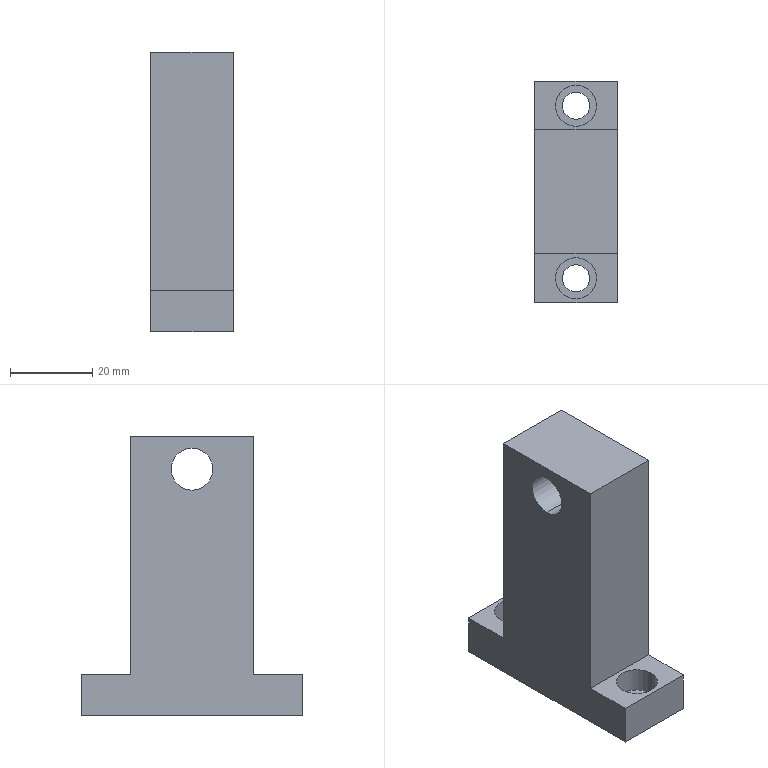Part | SolidWorks | features HoleWzd 2, Extrusion 1, ICE 1 | 1 solid | 22 faces | box 20 x 54 x 68 mm | volume 42750 mm3 | plane 12 | cylinder 10 | commonest cylinder face diameters 6.6 x4 10 x4 10.2 x2
STEP:
#1=CARTESIAN_POINT('',(-16.388,2.618,65.1));
#2=VERTEX_POINT('',#1);
#3=CARTESIAN_POINT('',(-16.388,2.618,54.9));
#4=VERTEX_POINT('',#3);
#5=CARTESIAN_POINT('',(-16.388,2.618,60.));
#6=DIRECTION('',(1.,0.,0.));
#7=DIRECTION('',(0.,1.,0.));
#8=AXIS2_PLACEMENT_3D('',#5,#6,#7);
#9=CIRCLE('',#8,5.1);
#10=EDGE_CURVE('',#2,#4,#9,.T.);
#11=ORIENTED_EDGE('',*,*,#10,.T.);
#12=CARTESIAN_POINT('',(-36.388,2.618,54.9));
#13=VERTEX_POINT('',#12);
#14=CARTESIAN_POINT('',(-36.388,2.618,54.9));
#15=DIRECTION('',(-1.,0.,0.));
#16=VECTOR('',#15,1000.);
#17=LINE('',#14,#16);
#18=EDGE_CURVE('',#4,#13,#17,.T.);
#19=ORIENTED_EDGE('',*,*,#18,.T.);
#20=CARTESIAN_POINT('',(-36.388,2.618,65.1));
#21=VERTEX_POINT('',#20);
#22=CARTESIAN_POINT('',(-36.388,2.618,60.));
#23=DIRECTION('',(-1.,0.,0.));
#24=DIRECTION('',(0.,0.,1.));
#25=AXIS2_PLACEMENT_3D('',#22,#23,#24);
#26=CIRCLE('',#25,5.1);
#27=EDGE_CURVE('',#13,#21,#26,.T.);
#28=ORIENTED_EDGE('',*,*,#27,.T.);
#29=CARTESIAN_POINT('',(-36.388,2.618,65.1));
#30=DIRECTION('',(-1.,0.,0.));
#31=VECTOR('',#30,1000.);
#32=LINE('',#29,#31);
#33=EDGE_CURVE('',#2,#21,#32,.T.);
#34=ORIENTED_EDGE('',*,*,#33,.F.);
#35=EDGE_LOOP('',(#11,#19,#28,#34));
#36=FACE_OUTER_BOUND('',#35,.T.);
#37=CARTESIAN_POINT('',(-36.388,2.618,60.));
#38=DIRECTION('',(-1.,0.,0.));
#39=DIRECTION('',(0.,0.,1.));
#40=AXIS2_PLACEMENT_3D('',#37,#38,#39);
#41=CYLINDRICAL_SURFACE('',#40,5.1);
#42=ADVANCED_FACE('',(#36),#41,.F.);
#43=CARTESIAN_POINT('',(-31.388,23.618,4.));
#44=VERTEX_POINT('',#43);
#45=CARTESIAN_POINT('',(-21.388,23.618,4.));
#46=VERTEX_POINT('',#45);
#47=CARTESIAN_POINT('',(-26.388,23.618,4.));
#48=DIRECTION('',(0.,0.,1.));
#49=DIRECTION('',(1.,0.,0.));
#50=AXIS2_PLACEMENT_3D('',#47,#48,#49);
#51=CIRCLE('',#50,5.);
#52=EDGE_CURVE('',#44,#46,#51,.T.);
#53=ORIENTED_EDGE('',*,*,#52,.F.);
#54=CARTESIAN_POINT('',(-31.388,23.618,10.));
#55=VERTEX_POINT('',#54);
#56=CARTESIAN_POINT('',(-31.388,23.618,10.));
#57=DIRECTION('',(0.,0.,1.));
#58=VECTOR('',#57,1000.);
#59=LINE('',#56,#58);
#60=EDGE_CURVE('',#44,#55,#59,.T.);
#61=ORIENTED_EDGE('',*,*,#60,.T.);
#62=CARTESIAN_POINT('',(-21.388,23.618,10.));
#63=VERTEX_POINT('',#62);
#64=CARTESIAN_POINT('',(-26.388,23.618,10.));
#65=DIRECTION('',(0.,0.,1.));
#66=DIRECTION('',(1.,0.,0.));
#67=AXIS2_PLACEMENT_3D('',#64,#65,#66);
#68=CIRCLE('',#67,5.);
#69=EDGE_CURVE('',#55,#63,#68,.T.);
#70=ORIENTED_EDGE('',*,*,#69,.T.);
#71=CARTESIAN_POINT('',(-21.388,23.618,10.));
#72=DIRECTION('',(0.,0.,1.));
#73=VECTOR('',#72,1000.);
#74=LINE('',#71,#73);
#75=EDGE_CURVE('',#46,#63,#74,.T.);
#76=ORIENTED_EDGE('',*,*,#75,.F.);
#77=EDGE_LOOP('',(#53,#61,#70,#76));
#78=FACE_OUTER_BOUND('',#77,.T.);
#79=CARTESIAN_POINT('',(-26.388,23.618,10.));
#80=DIRECTION('',(0.,0.,1.));
#81=DIRECTION('',(1.,0.,0.));
#82=AXIS2_PLACEMENT_3D('',#79,#80,#81);
#83=CYLINDRICAL_SURFACE('',#82,5.);
#84=ADVANCED_FACE('',(#78),#83,.F.);
#85=CARTESIAN_POINT('',(-29.688,23.618,0.));
#86=VERTEX_POINT('',#85);
#87=CARTESIAN_POINT('',(-23.088,23.618,0.));
#88=VERTEX_POINT('',#87);
#89=CARTESIAN_POINT('',(-26.388,23.618,0.));
#90=DIRECTION('',(0.,0.,1.));
#91=DIRECTION('',(1.,0.,0.));
#92=AXIS2_PLACEMENT_3D('',#89,#90,#91);
#93=CIRCLE('',#92,3.3);
#94=EDGE_CURVE('',#86,#88,#93,.T.);
#95=ORIENTED_EDGE('',*,*,#94,.F.);
#96=CARTESIAN_POINT('',(-29.688,23.618,4.));
#97=VERTEX_POINT('',#96);
#98=CARTESIAN_POINT('',(-29.688,23.618,10.));
#99=DIRECTION('',(0.,0.,1.));
#100=VECTOR('',#99,1000.);
#101=LINE('',#98,#100);
#102=EDGE_CURVE('',#86,#97,#101,.T.);
#103=ORIENTED_EDGE('',*,*,#102,.T.);
#104=CARTESIAN_POINT('',(-23.088,23.618,4.));
#105=VERTEX_POINT('',#104);
#106=CARTESIAN_POINT('',(-26.388,23.618,4.));
#107=DIRECTION('',(0.,0.,1.));
#108=DIRECTION('',(1.,0.,0.));
#109=AXIS2_PLACEMENT_3D('',#106,#107,#108);
#110=CIRCLE('',#109,3.3);
#111=EDGE_CURVE('',#97,#105,#110,.T.);
#112=ORIENTED_EDGE('',*,*,#111,.T.);
#113=CARTESIAN_POINT('',(-23.088,23.618,10.));
#114=DIRECTION('',(0.,0.,1.));
#115=VECTOR('',#114,1000.);
#116=LINE('',#113,#115);
#117=EDGE_CURVE('',#88,#105,#116,.T.);
#118=ORIENTED_EDGE('',*,*,#117,.F.);
#119=EDGE_LOOP('',(#95,#103,#112,#118));
#120=FACE_OUTER_BOUND('',#119,.T.);
#121=CARTESIAN_POINT('',(-26.388,23.618,10.));
#122=DIRECTION('',(0.,0.,1.));
#123=DIRECTION('',(1.,0.,0.));
#124=AXIS2_PLACEMENT_3D('',#121,#122,#123);
#125=CYLINDRICAL_SURFACE('',#124,3.3);
#126=ADVANCED_FACE('',(#120),#125,.F.);
#127=CARTESIAN_POINT('',(-31.388,-18.382,4.));
#128=VERTEX_POINT('',#127);
#129=CARTESIAN_POINT('',(-21.388,-18.382,4.));
#130=VERTEX_POINT('',#129);
#131=CARTESIAN_POINT('',(-26.388,-18.382,4.));
#132=DIRECTION('',(0.,0.,1.));
#133=DIRECTION('',(1.,0.,0.));
#134=AXIS2_PLACEMENT_3D('',#131,#132,#133);
#135=CIRCLE('',#134,5.);
#136=EDGE_CURVE('',#128,#130,#135,.T.);
#137=ORIENTED_EDGE('',*,*,#136,.F.);
#138=CARTESIAN_POINT('',(-31.388,-18.382,10.));
#139=VERTEX_POINT('',#138);
#140=CARTESIAN_POINT('',(-31.388,-18.382,10.));
#141=DIRECTION('',(0.,0.,1.));
#142=VECTOR('',#141,1000.);
#143=LINE('',#140,#142);
#144=EDGE_CURVE('',#128,#139,#143,.T.);
#145=ORIENTED_EDGE('',*,*,#144,.T.);
#146=CARTESIAN_POINT('',(-21.388,-18.382,10.));
#147=VERTEX_POINT('',#146);
#148=CARTESIAN_POINT('',(-26.388,-18.382,10.));
#149=DIRECTION('',(0.,0.,1.));
#150=DIRECTION('',(1.,0.,0.));
#151=AXIS2_PLACEMENT_3D('',#148,#149,#150);
#152=CIRCLE('',#151,5.);
#153=EDGE_CURVE('',#139,#147,#152,.T.);
#154=ORIENTED_EDGE('',*,*,#153,.T.);
#155=CARTESIAN_POINT('',(-21.388,-18.382,10.));
#156=DIRECTION('',(0.,0.,1.));
#157=VECTOR('',#156,1000.);
#158=LINE('',#155,#157);
#159=EDGE_CURVE('',#130,#147,#158,.T.);
#160=ORIENTED_EDGE('',*,*,#159,.F.);
#161=EDGE_LOOP('',(#137,#145,#154,#160));
#162=FACE_OUTER_BOUND('',#161,.T.);
#163=CARTESIAN_POINT('',(-26.388,-18.382,10.));
#164=DIRECTION('',(0.,0.,1.));
#165=DIRECTION('',(1.,0.,0.));
#166=AXIS2_PLACEMENT_3D('',#163,#164,#165);
#167=CYLINDRICAL_SURFACE('',#166,5.);
#168=ADVANCED_FACE('',(#162),#167,.F.);
#169=CARTESIAN_POINT('',(-29.688,-18.382,0.));
#170=VERTEX_POINT('',#169);
#171=CARTESIAN_POINT('',(-23.088,-18.382,0.));
#172=VERTEX_POINT('',#171);
#173=CARTESIAN_POINT('',(-26.388,-18.382,0.));
#174=DIRECTION('',(0.,0.,1.));
#175=DIRECTION('',(1.,0.,0.));
#176=AXIS2_PLACEMENT_3D('',#173,#174,#175);
#177=CIRCLE('',#176,3.3);
#178=EDGE_CURVE('',#170,#172,#177,.T.);
#179=ORIENTED_EDGE('',*,*,#178,.F.);
#180=CARTESIAN_POINT('',(-29.688,-18.382,4.));
#181=VERTEX_POINT('',#180);
#182=CARTESIAN_POINT('',(-29.688,-18.382,10.));
#183=DIRECTION('',(0.,0.,1.));
#184=VECTOR('',#183,1000.);
#185=LINE('',#182,#184);
#186=EDGE_CURVE('',#170,#181,#185,.T.);
#187=ORIENTED_EDGE('',*,*,#186,.T.);
#188=CARTESIAN_POINT('',(-23.088,-18.382,4.));
#189=VERTEX_POINT('',#188);
#190=CARTESIAN_POINT('',(-26.388,-18.382,4.));
#191=DIRECTION('',(0.,0.,1.));
#192=DIRECTION('',(1.,0.,0.));
#193=AXIS2_PLACEMENT_3D('',#190,#191,#192);
#194=CIRCLE('',#193,3.3);
#195=EDGE_CURVE('',#181,#189,#194,.T.);
#196=ORIENTED_EDGE('',*,*,#195,.T.);
#197=CARTESIAN_POINT('',(-23.088,-18.382,10.));
#198=DIRECTION('',(0.,0.,1.));
#199=VECTOR('',#198,1000.);
#200=LINE('',#197,#199);
#201=EDGE_CURVE('',#172,#189,#200,.T.);
#202=ORIENTED_EDGE('',*,*,#201,.F.);
#203=EDGE_LOOP('',(#179,#187,#196,#202));
#204=FACE_OUTER_BOUND('',#203,.T.);
#205=CARTESIAN_POINT('',(-26.388,-18.382,10.));
#206=DIRECTION('',(0.,0.,1.));
#207=DIRECTION('',(1.,0.,0.));
#208=AXIS2_PLACEMENT_3D('',#205,#206,#207);
#209=CYLINDRICAL_SURFACE('',#208,3.3);
#210=ADVANCED_FACE('',(#204),#209,.F.);
#211=CARTESIAN_POINT('',(-26.388,23.618,10.));
#212=DIRECTION('',(0.,0.,1.));
#213=DIRECTION('',(1.,0.,0.));
#214=AXIS2_PLACEMENT_3D('',#211,#212,#213);
#215=CIRCLE('',#214,5.);
#216=EDGE_CURVE('',#63,#55,#215,.T.);
#217=ORIENTED_EDGE('',*,*,#216,.F.);
#218=ORIENTED_EDGE('',*,*,#69,.F.);
#219=EDGE_LOOP('',(#217,#218));
#220=FACE_BOUND('',#219,.T.);
#221=CARTESIAN_POINT('',(-16.388,17.618,10.));
#222=VERTEX_POINT('',#221);
#223=CARTESIAN_POINT('',(-36.388,17.618,10.));
#224=VERTEX_POINT('',#223);
#225=CARTESIAN_POINT('',(-36.388,17.618,10.));
#226=DIRECTION('',(-1.,0.,0.));
#227=VECTOR('',#226,1000.);
#228=LINE('',#225,#227);
#229=EDGE_CURVE('',#222,#224,#228,.T.);
#230=ORIENTED_EDGE('',*,*,#229,.F.);
#231=CARTESIAN_POINT('',(-16.388,29.618,10.));
#232=VERTEX_POINT('',#231);
#233=CARTESIAN_POINT('',(-16.388,29.618,10.));
#234=DIRECTION('',(0.,-1.,0.));
#235=VECTOR('',#234,1000.);
#236=LINE('',#233,#235);
#237=EDGE_CURVE('',#232,#222,#236,.T.);
#238=ORIENTED_EDGE('',*,*,#237,.F.);
#239=CARTESIAN_POINT('',(-36.388,29.618,10.));
#240=VERTEX_POINT('',#239);
#241=CARTESIAN_POINT('',(-36.388,29.618,10.));
#242=DIRECTION('',(1.,0.,0.));
#243=VECTOR('',#242,1000.);
#244=LINE('',#241,#243);
#245=EDGE_CURVE('',#240,#232,#244,.T.);
#246=ORIENTED_EDGE('',*,*,#245,.F.);
#247=CARTESIAN_POINT('',(-36.388,29.618,10.));
#248=DIRECTION('',(0.,-1.,0.));
#249=VECTOR('',#248,1000.);
#250=LINE('',#247,#249);
#251=EDGE_CURVE('',#240,#224,#250,.T.);
#252=ORIENTED_EDGE('',*,*,#251,.T.);
#253=EDGE_LOOP('',(#230,#238,#246,#252));
#254=FACE_OUTER_BOUND('',#253,.T.);
#255=CARTESIAN_POINT('',(0.,0.,10.));
#256=DIRECTION('',(0.,0.,-1.));
#257=DIRECTION('',(-1.,0.,0.));
#258=AXIS2_PLACEMENT_3D('',#255,#256,#257);
#259=PLANE('',#258);
#260=ADVANCED_FACE('',(#220,#254),#259,.F.);
#261=CARTESIAN_POINT('',(-26.388,-18.382,10.));
#262=DIRECTION('',(0.,0.,1.));
#263=DIRECTION('',(1.,0.,0.));
#264=AXIS2_PLACEMENT_3D('',#261,#262,#263);
#265=CIRCLE('',#264,5.);
#266=EDGE_CURVE('',#147,#139,#265,.T.);
#267=ORIENTED_EDGE('',*,*,#266,.F.);
#268=ORIENTED_EDGE('',*,*,#153,.F.);
#269=EDGE_LOOP('',(#267,#268));
#270=FACE_BOUND('',#269,.T.);
#271=CARTESIAN_POINT('',(-36.388,-12.382,10.));
#272=VERTEX_POINT('',#271);
#273=CARTESIAN_POINT('',(-16.388,-12.382,10.));
#274=VERTEX_POINT('',#273);
#275=CARTESIAN_POINT('',(-36.388,-12.382,10.));
#276=DIRECTION('',(1.,0.,0.));
#277=VECTOR('',#276,1000.);
#278=LINE('',#275,#277);
#279=EDGE_CURVE('',#272,#274,#278,.T.);
#280=ORIENTED_EDGE('',*,*,#279,.F.);
#281=CARTESIAN_POINT('',(-36.388,-24.382,10.));
#282=VERTEX_POINT('',#281);
#283=CARTESIAN_POINT('',(-36.388,29.618,10.));
#284=DIRECTION('',(0.,-1.,0.));
#285=VECTOR('',#284,1000.);
#286=LINE('',#283,#285);
#287=EDGE_CURVE('',#272,#282,#286,.T.);
#288=ORIENTED_EDGE('',*,*,#287,.T.);
#289=CARTESIAN_POINT('',(-16.388,-24.382,10.));
#290=VERTEX_POINT('',#289);
#291=CARTESIAN_POINT('',(-36.388,-24.382,10.));
#292=DIRECTION('',(1.,0.,0.));
#293=VECTOR('',#292,1000.);
#294=LINE('',#291,#293);
#295=EDGE_CURVE('',#282,#290,#294,.T.);
#296=ORIENTED_EDGE('',*,*,#295,.T.);
#297=CARTESIAN_POINT('',(-16.388,29.618,10.));
#298=DIRECTION('',(0.,-1.,0.));
#299=VECTOR('',#298,1000.);
#300=LINE('',#297,#299);
#301=EDGE_CURVE('',#274,#290,#300,.T.);
#302=ORIENTED_EDGE('',*,*,#301,.F.);
#303=EDGE_LOOP('',(#280,#288,#296,#302));
#304=FACE_OUTER_BOUND('',#303,.T.);
#305=CARTESIAN_POINT('',(0.,0.,10.));
#306=DIRECTION('',(0.,0.,-1.));
#307=DIRECTION('',(-1.,0.,0.));
#308=AXIS2_PLACEMENT_3D('',#305,#306,#307);
#309=PLANE('',#308);
#310=ADVANCED_FACE('',(#270,#304),#309,.F.);
#311=CARTESIAN_POINT('',(-36.388,29.618,0.));
#312=VERTEX_POINT('',#311);
#313=CARTESIAN_POINT('',(-16.388,29.618,0.));
#314=VERTEX_POINT('',#313);
#315=CARTESIAN_POINT('',(-36.388,29.618,0.));
#316=DIRECTION('',(1.,0.,0.));
#317=VECTOR('',#316,1000.);
#318=LINE('',#315,#317);
#319=EDGE_CURVE('',#312,#314,#318,.T.);
#320=ORIENTED_EDGE('',*,*,#319,.F.);
#321=CARTESIAN_POINT('',(-36.388,29.618,10.));
#322=DIRECTION('',(0.,0.,-1.));
#323=VECTOR('',#322,1000.);
#324=LINE('',#321,#323);
#325=EDGE_CURVE('',#240,#312,#324,.T.);
#326=ORIENTED_EDGE('',*,*,#325,.F.);
#327=ORIENTED_EDGE('',*,*,#245,.T.);
#328=CARTESIAN_POINT('',(-16.388,29.618,10.));
#329=DIRECTION('',(0.,0.,-1.));
#330=VECTOR('',#329,1000.);
#331=LINE('',#328,#330);
#332=EDGE_CURVE('',#232,#314,#331,.T.);
#333=ORIENTED_EDGE('',*,*,#332,.T.);
#334=EDGE_LOOP('',(#320,#326,#327,#333));
#335=FACE_OUTER_BOUND('',#334,.T.);
#336=CARTESIAN_POINT('',(-36.388,29.618,10.));
#337=DIRECTION('',(0.,1.,0.));
#338=DIRECTION('',(0.,0.,1.));
#339=AXIS2_PLACEMENT_3D('',#336,#337,#338);
#340=PLANE('',#339);
#341=ADVANCED_FACE('',(#335),#340,.T.);
#342=CARTESIAN_POINT('',(-36.388,2.618,60.));
#343=DIRECTION('',(-1.,0.,0.));
#344=DIRECTION('',(0.,0.,1.));
#345=AXIS2_PLACEMENT_3D('',#342,#343,#344);
#346=CIRCLE('',#345,5.1);
#347=EDGE_CURVE('',#21,#13,#346,.T.);
#348=ORIENTED_EDGE('',*,*,#347,.F.);
#349=ORIENTED_EDGE('',*,*,#27,.F.);
#350=EDGE_LOOP('',(#348,#349));
#351=FACE_BOUND('',#350,.T.);
#352=CARTESIAN_POINT('',(-36.388,-24.382,0.));
#353=VERTEX_POINT('',#352);
#354=CARTESIAN_POINT('',(-36.388,29.618,0.));
#355=DIRECTION('',(0.,-1.,0.));
#356=VECTOR('',#355,1000.);
#357=LINE('',#354,#356);
#358=EDGE_CURVE('',#312,#353,#357,.T.);
#359=ORIENTED_EDGE('',*,*,#358,.T.);
#360=CARTESIAN_POINT('',(-36.388,-24.382,10.));
#361=DIRECTION('',(0.,0.,-1.));
#362=VECTOR('',#361,1000.);
#363=LINE('',#360,#362);
#364=EDGE_CURVE('',#282,#353,#363,.T.);
#365=ORIENTED_EDGE('',*,*,#364,.F.);
#366=ORIENTED_EDGE('',*,*,#287,.F.);
#367=CARTESIAN_POINT('',(-36.388,-12.382,68.));
#368=VERTEX_POINT('',#367);
#369=CARTESIAN_POINT('',(-36.388,-12.382,68.));
#370=DIRECTION('',(0.,0.,-1.));
#371=VECTOR('',#370,1000.);
#372=LINE('',#369,#371);
#373=EDGE_CURVE('',#368,#272,#372,.T.);
#374=ORIENTED_EDGE('',*,*,#373,.F.);
#375=CARTESIAN_POINT('',(-36.388,17.618,68.));
#376=VERTEX_POINT('',#375);
#377=CARTESIAN_POINT('',(-36.388,17.618,68.));
#378=DIRECTION('',(0.,-1.,0.));
#379=VECTOR('',#378,1000.);
#380=LINE('',#377,#379);
#381=EDGE_CURVE('',#376,#368,#380,.T.);
#382=ORIENTED_EDGE('',*,*,#381,.F.);
#383=CARTESIAN_POINT('',(-36.388,17.618,68.));
#384=DIRECTION('',(0.,0.,-1.));
#385=VECTOR('',#384,1000.);
#386=LINE('',#383,#385);
#387=EDGE_CURVE('',#376,#224,#386,.T.);
#388=ORIENTED_EDGE('',*,*,#387,.T.);
#389=ORIENTED_EDGE('',*,*,#251,.F.);
#390=ORIENTED_EDGE('',*,*,#325,.T.);
#391=EDGE_LOOP('',(#359,#365,#366,#374,#382,#388,#389,#390));
#392=FACE_OUTER_BOUND('',#391,.T.);
#393=CARTESIAN_POINT('',(-36.388,29.618,10.));
#394=DIRECTION('',(1.,0.,0.));
#395=DIRECTION('',(0.,1.,0.));
#396=AXIS2_PLACEMENT_3D('',#393,#394,#395);
#397=PLANE('',#396);
#398=ADVANCED_FACE('',(#351,#392),#397,.F.);
#399=CARTESIAN_POINT('',(-16.388,-24.382,0.));
#400=VERTEX_POINT('',#399);
#401=CARTESIAN_POINT('',(-36.388,-24.382,0.));
#402=DIRECTION('',(1.,0.,0.));
#403=VECTOR('',#402,1000.);
#404=LINE('',#401,#403);
#405=EDGE_CURVE('',#353,#400,#404,.T.);
#406=ORIENTED_EDGE('',*,*,#405,.T.);
#407=CARTESIAN_POINT('',(-16.388,-24.382,10.));
#408=DIRECTION('',(0.,0.,-1.));
#409=VECTOR('',#408,1000.);
#410=LINE('',#407,#409);
#411=EDGE_CURVE('',#290,#400,#410,.T.);
#412=ORIENTED_EDGE('',*,*,#411,.F.);
#413=ORIENTED_EDGE('',*,*,#295,.F.);
#414=ORIENTED_EDGE('',*,*,#364,.T.);
#415=EDGE_LOOP('',(#406,#412,#413,#414));
#416=FACE_OUTER_BOUND('',#415,.T.);
#417=CARTESIAN_POINT('',(-36.388,-24.382,10.));
#418=DIRECTION('',(0.,1.,0.));
#419=DIRECTION('',(0.,0.,1.));
#420=AXIS2_PLACEMENT_3D('',#417,#418,#419);
#421=PLANE('',#420);
#422=ADVANCED_FACE('',(#416),#421,.F.);
#423=ORIENTED_EDGE('',*,*,#10,.F.);
#424=CARTESIAN_POINT('',(-16.388,2.618,60.));
#425=DIRECTION('',(1.,0.,0.));
#426=DIRECTION('',(0.,1.,0.));
#427=AXIS2_PLACEMENT_3D('',#424,#425,#426);
#428=CIRCLE('',#427,5.1);
#429=EDGE_CURVE('',#4,#2,#428,.T.);
#430=ORIENTED_EDGE('',*,*,#429,.F.);
#431=EDGE_LOOP('',(#423,#430));
#432=FACE_BOUND('',#431,.T.);
#433=CARTESIAN_POINT('',(-16.388,29.618,0.));
#434=DIRECTION('',(0.,-1.,0.));
#435=VECTOR('',#434,1000.);
#436=LINE('',#433,#435);
#437=EDGE_CURVE('',#314,#400,#436,.T.);
#438=ORIENTED_EDGE('',*,*,#437,.F.);
#439=ORIENTED_EDGE('',*,*,#332,.F.);
#440=ORIENTED_EDGE('',*,*,#237,.T.);
#441=CARTESIAN_POINT('',(-16.388,17.618,68.));
#442=VERTEX_POINT('',#441);
#443=CARTESIAN_POINT('',(-16.388,17.618,68.));
#444=DIRECTION('',(0.,0.,-1.));
#445=VECTOR('',#444,1000.);
#446=LINE('',#443,#445);
#447=EDGE_CURVE('',#442,#222,#446,.T.);
#448=ORIENTED_EDGE('',*,*,#447,.F.);
#449=CARTESIAN_POINT('',(-16.388,-12.382,68.));
#450=VERTEX_POINT('',#449);
#451=CARTESIAN_POINT('',(-16.388,17.618,68.));
#452=DIRECTION('',(0.,1.,0.));
#453=VECTOR('',#452,1000.);
#454=LINE('',#451,#453);
#455=EDGE_CURVE('',#450,#442,#454,.T.);
#456=ORIENTED_EDGE('',*,*,#455,.F.);
#457=CARTESIAN_POINT('',(-16.388,-12.382,68.));
#458=DIRECTION('',(0.,0.,-1.));
#459=VECTOR('',#458,1000.);
#460=LINE('',#457,#459);
#461=EDGE_CURVE('',#450,#274,#460,.T.);
#462=ORIENTED_EDGE('',*,*,#461,.T.);
#463=ORIENTED_EDGE('',*,*,#301,.T.);
#464=ORIENTED_EDGE('',*,*,#411,.T.);
#465=EDGE_LOOP('',(#438,#439,#440,#448,#456,#462,#463,#464));
#466=FACE_OUTER_BOUND('',#465,.T.);
#467=CARTESIAN_POINT('',(-16.388,29.618,10.));
#468=DIRECTION('',(1.,0.,0.));
#469=DIRECTION('',(0.,1.,0.));
#470=AXIS2_PLACEMENT_3D('',#467,#468,#469);
#471=PLANE('',#470);
#472=ADVANCED_FACE('',(#432,#466),#471,.T.);
#473=CARTESIAN_POINT('',(-26.388,23.618,0.));
#474=DIRECTION('',(0.,0.,1.));
#475=DIRECTION('',(1.,0.,0.));
#476=AXIS2_PLACEMENT_3D('',#473,#474,#475);
#477=CIRCLE('',#476,3.3);
#478=EDGE_CURVE('',#88,#86,#477,.T.);
#479=ORIENTED_EDGE('',*,*,#478,.T.);
#480=ORIENTED_EDGE('',*,*,#94,.T.);
#481=EDGE_LOOP('',(#479,#480));
#482=FACE_BOUND('',#481,.T.);
#483=CARTESIAN_POINT('',(-26.388,-18.382,0.));
#484=DIRECTION('',(0.,0.,1.));
#485=DIRECTION('',(1.,0.,0.));
#486=AXIS2_PLACEMENT_3D('',#483,#484,#485);
#487=CIRCLE('',#486,3.3);
#488=EDGE_CURVE('',#172,#170,#487,.T.);
#489=ORIENTED_EDGE('',*,*,#488,.T.);
#490=ORIENTED_EDGE('',*,*,#178,.T.);
#491=EDGE_LOOP('',(#489,#490));
#492=FACE_BOUND('',#491,.T.);
#493=ORIENTED_EDGE('',*,*,#319,.T.);
#494=ORIENTED_EDGE('',*,*,#437,.T.);
#495=ORIENTED_EDGE('',*,*,#405,.F.);
#496=ORIENTED_EDGE('',*,*,#358,.F.);
#497=EDGE_LOOP('',(#493,#494,#495,#496));
#498=FACE_OUTER_BOUND('',#497,.T.);
#499=CARTESIAN_POINT('',(0.,0.,0.));
#500=DIRECTION('',(0.,0.,-1.));
#501=DIRECTION('',(-1.,0.,0.));
#502=AXIS2_PLACEMENT_3D('',#499,#500,#501);
#503=PLANE('',#502);
#504=ADVANCED_FACE('',(#482,#492,#498),#503,.T.);
#505=ORIENTED_EDGE('',*,*,#279,.T.);
#506=ORIENTED_EDGE('',*,*,#461,.F.);
#507=CARTESIAN_POINT('',(-36.388,-12.382,68.));
#508=DIRECTION('',(1.,0.,0.));
#509=VECTOR('',#508,1000.);
#510=LINE('',#507,#509);
#511=EDGE_CURVE('',#368,#450,#510,.T.);
#512=ORIENTED_EDGE('',*,*,#511,.F.);
#513=ORIENTED_EDGE('',*,*,#373,.T.);
#514=EDGE_LOOP('',(#505,#506,#512,#513));
#515=FACE_OUTER_BOUND('',#514,.T.);
#516=CARTESIAN_POINT('',(-36.388,-12.382,68.));
#517=DIRECTION('',(0.,1.,0.));
#518=DIRECTION('',(0.,0.,1.));
#519=AXIS2_PLACEMENT_3D('',#516,#517,#518);
#520=PLANE('',#519);
#521=ADVANCED_FACE('',(#515),#520,.F.);
#522=ORIENTED_EDGE('',*,*,#229,.T.);
#523=ORIENTED_EDGE('',*,*,#387,.F.);
#524=CARTESIAN_POINT('',(-36.388,17.618,68.));
#525=DIRECTION('',(-1.,0.,0.));
#526=VECTOR('',#525,1000.);
#527=LINE('',#524,#526);
#528=EDGE_CURVE('',#442,#376,#527,.T.);
#529=ORIENTED_EDGE('',*,*,#528,.F.);
#530=ORIENTED_EDGE('',*,*,#447,.T.);
#531=EDGE_LOOP('',(#522,#523,#529,#530));
#532=FACE_OUTER_BOUND('',#531,.T.);
#533=CARTESIAN_POINT('',(-36.388,17.618,68.));
#534=DIRECTION('',(0.,-1.,0.));
#535=DIRECTION('',(0.,0.,-1.));
#536=AXIS2_PLACEMENT_3D('',#533,#534,#535);
#537=PLANE('',#536);
#538=ADVANCED_FACE('',(#532),#537,.F.);
#539=ORIENTED_EDGE('',*,*,#381,.T.);
#540=ORIENTED_EDGE('',*,*,#511,.T.);
#541=ORIENTED_EDGE('',*,*,#455,.T.);
#542=ORIENTED_EDGE('',*,*,#528,.T.);
#543=EDGE_LOOP('',(#539,#540,#541,#542));
#544=FACE_OUTER_BOUND('',#543,.T.);
#545=CARTESIAN_POINT('',(0.,0.,68.));
#546=DIRECTION('',(0.,0.,1.));
#547=DIRECTION('',(1.,0.,0.));
#548=AXIS2_PLACEMENT_3D('',#545,#546,#547);
#549=PLANE('',#548);
#550=ADVANCED_FACE('',(#544),#549,.T.);
#551=ORIENTED_EDGE('',*,*,#186,.F.);
#552=ORIENTED_EDGE('',*,*,#488,.F.);
#553=ORIENTED_EDGE('',*,*,#201,.T.);
#554=CARTESIAN_POINT('',(-26.388,-18.382,4.));
#555=DIRECTION('',(0.,0.,1.));
#556=DIRECTION('',(1.,0.,0.));
#557=AXIS2_PLACEMENT_3D('',#554,#555,#556);
#558=CIRCLE('',#557,3.3);
#559=EDGE_CURVE('',#189,#181,#558,.T.);
#560=ORIENTED_EDGE('',*,*,#559,.T.);
#561=EDGE_LOOP('',(#551,#552,#553,#560));
#562=FACE_OUTER_BOUND('',#561,.T.);
#563=CARTESIAN_POINT('',(-26.388,-18.382,10.));
#564=DIRECTION('',(0.,0.,1.));
#565=DIRECTION('',(1.,0.,0.));
#566=AXIS2_PLACEMENT_3D('',#563,#564,#565);
#567=CYLINDRICAL_SURFACE('',#566,3.3);
#568=ADVANCED_FACE('',(#562),#567,.F.);
#569=ORIENTED_EDGE('',*,*,#559,.F.);
#570=ORIENTED_EDGE('',*,*,#195,.F.);
#571=EDGE_LOOP('',(#569,#570));
#572=FACE_BOUND('',#571,.T.);
#573=CARTESIAN_POINT('',(-26.388,-18.382,4.));
#574=DIRECTION('',(0.,0.,1.));
#575=DIRECTION('',(1.,0.,0.));
#576=AXIS2_PLACEMENT_3D('',#573,#574,#575);
#577=CIRCLE('',#576,5.);
#578=EDGE_CURVE('',#130,#128,#577,.T.);
#579=ORIENTED_EDGE('',*,*,#578,.T.);
#580=ORIENTED_EDGE('',*,*,#136,.T.);
#581=EDGE_LOOP('',(#579,#580));
#582=FACE_OUTER_BOUND('',#581,.T.);
#583=CARTESIAN_POINT('',(-23.088,-18.382,4.));
#584=DIRECTION('',(0.,0.,-1.));
#585=DIRECTION('',(-1.,0.,0.));
#586=AXIS2_PLACEMENT_3D('',#583,#584,#585);
#587=PLANE('',#586);
#588=ADVANCED_FACE('',(#572,#582),#587,.F.);
#589=ORIENTED_EDGE('',*,*,#144,.F.);
#590=ORIENTED_EDGE('',*,*,#578,.F.);
#591=ORIENTED_EDGE('',*,*,#159,.T.);
#592=ORIENTED_EDGE('',*,*,#266,.T.);
#593=EDGE_LOOP('',(#589,#590,#591,#592));
#594=FACE_OUTER_BOUND('',#593,.T.);
#595=CARTESIAN_POINT('',(-26.388,-18.382,10.));
#596=DIRECTION('',(0.,0.,1.));
#597=DIRECTION('',(1.,0.,0.));
#598=AXIS2_PLACEMENT_3D('',#595,#596,#597);
#599=CYLINDRICAL_SURFACE('',#598,5.);
#600=ADVANCED_FACE('',(#594),#599,.F.);
#601=ORIENTED_EDGE('',*,*,#102,.F.);
#602=ORIENTED_EDGE('',*,*,#478,.F.);
#603=ORIENTED_EDGE('',*,*,#117,.T.);
#604=CARTESIAN_POINT('',(-26.388,23.618,4.));
#605=DIRECTION('',(0.,0.,1.));
#606=DIRECTION('',(1.,0.,0.));
#607=AXIS2_PLACEMENT_3D('',#604,#605,#606);
#608=CIRCLE('',#607,3.3);
#609=EDGE_CURVE('',#105,#97,#608,.T.);
#610=ORIENTED_EDGE('',*,*,#609,.T.);
#611=EDGE_LOOP('',(#601,#602,#603,#610));
#612=FACE_OUTER_BOUND('',#611,.T.);
#613=CARTESIAN_POINT('',(-26.388,23.618,10.));
#614=DIRECTION('',(0.,0.,1.));
#615=DIRECTION('',(1.,0.,0.));
#616=AXIS2_PLACEMENT_3D('',#613,#614,#615);
#617=CYLINDRICAL_SURFACE('',#616,3.3);
#618=ADVANCED_FACE('',(#612),#617,.F.);
#619=ORIENTED_EDGE('',*,*,#609,.F.);
#620=ORIENTED_EDGE('',*,*,#111,.F.);
#621=EDGE_LOOP('',(#619,#620));
#622=FACE_BOUND('',#621,.T.);
#623=CARTESIAN_POINT('',(-26.388,23.618,4.));
#624=DIRECTION('',(0.,0.,1.));
#625=DIRECTION('',(1.,0.,0.));
#626=AXIS2_PLACEMENT_3D('',#623,#624,#625);
#627=CIRCLE('',#626,5.);
#628=EDGE_CURVE('',#46,#44,#627,.T.);
#629=ORIENTED_EDGE('',*,*,#628,.T.);
#630=ORIENTED_EDGE('',*,*,#52,.T.);
#631=EDGE_LOOP('',(#629,#630));
#632=FACE_OUTER_BOUND('',#631,.T.);
#633=CARTESIAN_POINT('',(-23.088,23.618,4.));
#634=DIRECTION('',(0.,0.,-1.));
#635=DIRECTION('',(-1.,0.,0.));
#636=AXIS2_PLACEMENT_3D('',#633,#634,#635);
#637=PLANE('',#636);
#638=ADVANCED_FACE('',(#622,#632),#637,.F.);
#639=ORIENTED_EDGE('',*,*,#60,.F.);
#640=ORIENTED_EDGE('',*,*,#628,.F.);
#641=ORIENTED_EDGE('',*,*,#75,.T.);
#642=ORIENTED_EDGE('',*,*,#216,.T.);
#643=EDGE_LOOP('',(#639,#640,#641,#642));
#644=FACE_OUTER_BOUND('',#643,.T.);
#645=CARTESIAN_POINT('',(-26.388,23.618,10.));
#646=DIRECTION('',(0.,0.,1.));
#647=DIRECTION('',(1.,0.,0.));
#648=AXIS2_PLACEMENT_3D('',#645,#646,#647);
#649=CYLINDRICAL_SURFACE('',#648,5.);
#650=ADVANCED_FACE('',(#644),#649,.F.);
#651=ORIENTED_EDGE('',*,*,#18,.F.);
#652=ORIENTED_EDGE('',*,*,#429,.T.);
#653=ORIENTED_EDGE('',*,*,#33,.T.);
#654=ORIENTED_EDGE('',*,*,#347,.T.);
#655=EDGE_LOOP('',(#651,#652,#653,#654));
#656=FACE_OUTER_BOUND('',#655,.T.);
#657=CARTESIAN_POINT('',(-36.388,2.618,60.));
#658=DIRECTION('',(-1.,0.,0.));
#659=DIRECTION('',(0.,0.,1.));
#660=AXIS2_PLACEMENT_3D('',#657,#658,#659);
#661=CYLINDRICAL_SURFACE('',#660,5.1);
#662=ADVANCED_FACE('',(#656),#661,.F.);
#663=CLOSED_SHELL('',(#42,#84,#126,#168,#210,#260,#310,#341,#398,#422,#472,#504,#521,#538,#550,#568,#588,#600,#618,#638,#650,#662));
#664=MANIFOLD_SOLID_BREP('',#663);
#665=CARTESIAN_POINT('',(0.,0.,0.));
#666=DIRECTION('',(0.,0.,1.));
#667=DIRECTION('',(1.,0.,0.));
#668=AXIS2_PLACEMENT_3D('',#665,#666,#667);
#669=(LENGTH_UNIT()NAMED_UNIT(*)SI_UNIT(.MILLI.,.METRE.));
#670=UNCERTAINTY_MEASURE_WITH_UNIT(LENGTH_MEASURE(0.00001),#669,'','');
#671=(NAMED_UNIT(*)PLANE_ANGLE_UNIT()SI_UNIT($,.RADIAN.));
#672=(NAMED_UNIT(*)SI_UNIT($,.STERADIAN.)SOLID_ANGLE_UNIT());
#673=(GEOMETRIC_REPRESENTATION_CONTEXT(3)GLOBAL_UNCERTAINTY_ASSIGNED_CONTEXT((#670))GLOBAL_UNIT_ASSIGNED_CONTEXT((#669,#671,#672))REPRESENTATION_CONTEXT('',''));
#674=ADVANCED_BREP_SHAPE_REPRESENTATION('',(#664,#668),#673);